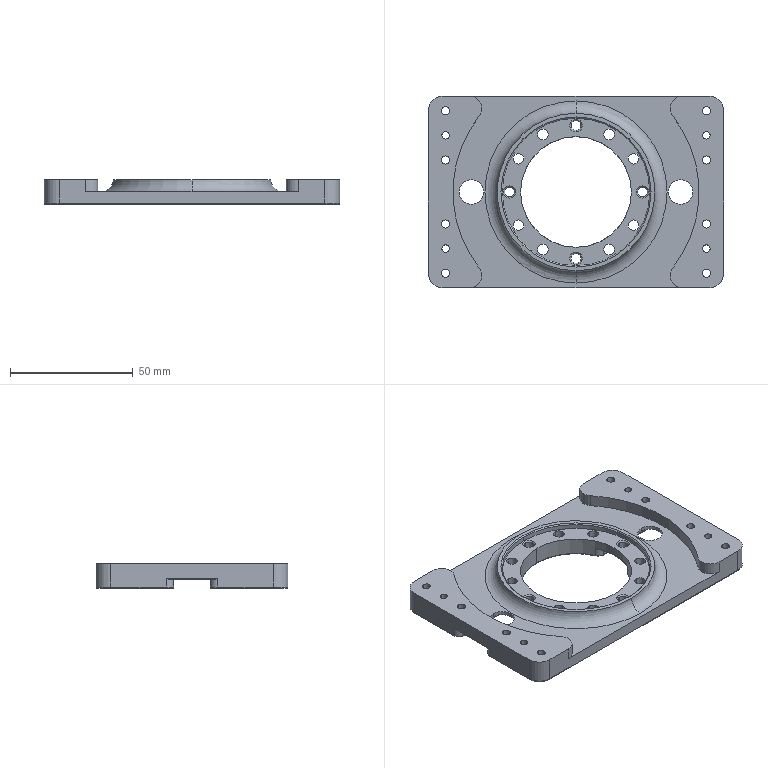NC program | NX | posted with a generic post | part box 120 x 78 x 10 mm
Lines 1 to 34 of 8419:
N10 G17 G21 G94 G90
(FLOOR_WALL_COPY_1 , TOOL : D80)
N12 T19 M6
N14 G54
N16 G17 G0 G90 X-105. Y38.997 B0. C0. S6500 M3
N18 G43 Z30. H19
N20 Z4.
N22 G94 G1 Z1. F1500.
N24 X-100.
N26 X100.
N28 Y15.999
N30 X-100.
N32 Y-7.
N34 X100.
N36 X105.
N38 Z4.
N40 G0 Z30.
N42 X-105. Y38.997
N44 Z3.
N46 G1 Z0.
N48 X-100.
N50 X100.
N52 Y15.999
N54 X-100.
N56 Y-7.
N58 X100.
N60 X105.
N62 Z3.
N64 G0 Z30.
N66 M5